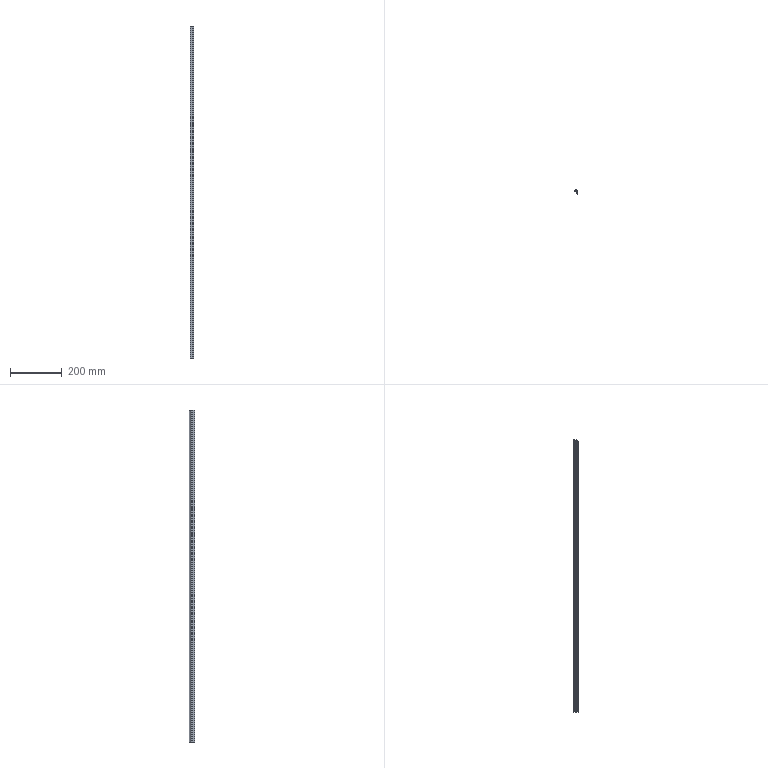Part | SolidWorks | features BaseBody 1, ICE 1, MoveFace 1 | 1 solid | 27 faces | box 14 x 20.3 x 1280 mm | volume 65172 mm3 | plane 20 | cylinder 7 | commonest cylinder face diameters 0.387 x2 0.8 x2 0.4 x1 20 x1 22 x1
STEP:
#1=CARTESIAN_POINT('',(-5.304,-0.625,200.));
#2=VERTEX_POINT('',#1);
#3=CARTESIAN_POINT('',(-5.449,-0.8125,200.));
#4=VERTEX_POINT('',#3);
#5=CARTESIAN_POINT('',(-5.255,-0.8125,200.));
#6=DIRECTION('',(0.,0.,1.));
#7=DIRECTION('',(-1.,0.,0.));
#8=AXIS2_PLACEMENT_3D('',#5,#6,#7);
#9=CIRCLE('',#8,0.1937);
#10=EDGE_CURVE('',#2,#4,#9,.T.);
#11=ORIENTED_EDGE('',*,*,#10,.T.);
#12=CARTESIAN_POINT('',(-5.449,-0.8125,-1080.));
#13=VERTEX_POINT('',#12);
#14=CARTESIAN_POINT('',(-5.449,-0.8125,230.));
#15=DIRECTION('',(0.,0.,-1.));
#16=VECTOR('',#15,1000.);
#17=LINE('',#14,#16);
#18=EDGE_CURVE('',#4,#13,#17,.T.);
#19=ORIENTED_EDGE('',*,*,#18,.T.);
#20=CARTESIAN_POINT('',(-5.304,-0.625,-1080.));
#21=VERTEX_POINT('',#20);
#22=CARTESIAN_POINT('',(-5.255,-0.8125,-1080.));
#23=DIRECTION('',(0.,0.,-1.));
#24=DIRECTION('',(1.,0.,0.));
#25=AXIS2_PLACEMENT_3D('',#22,#23,#24);
#26=CIRCLE('',#25,0.1937);
#27=EDGE_CURVE('',#13,#21,#26,.T.);
#28=ORIENTED_EDGE('',*,*,#27,.T.);
#29=CARTESIAN_POINT('',(-5.304,-0.625,230.));
#30=DIRECTION('',(0.,0.,-1.));
#31=VECTOR('',#30,1000.);
#32=LINE('',#29,#31);
#33=EDGE_CURVE('',#2,#21,#32,.T.);
#34=ORIENTED_EDGE('',*,*,#33,.F.);
#35=EDGE_LOOP('',(#11,#19,#28,#34));
#36=FACE_OUTER_BOUND('',#35,.T.);
#37=CARTESIAN_POINT('',(-5.255,-0.8125,230.));
#38=DIRECTION('',(0.,0.,-1.));
#39=DIRECTION('',(-1.,0.,0.));
#40=AXIS2_PLACEMENT_3D('',#37,#38,#39);
#41=CYLINDRICAL_SURFACE('',#40,0.1937);
#42=ADVANCED_FACE('',(#36),#41,.F.);
#43=CARTESIAN_POINT('',(5.,-1.,-1080.));
#44=VERTEX_POINT('',#43);
#45=CARTESIAN_POINT('',(5.,-14.3,-1080.));
#46=VERTEX_POINT('',#45);
#47=CARTESIAN_POINT('',(5.,29.623,-1080.));
#48=DIRECTION('',(0.,-1.,0.));
#49=VECTOR('',#48,1000.);
#50=LINE('',#47,#49);
#51=EDGE_CURVE('',#44,#46,#50,.T.);
#52=ORIENTED_EDGE('',*,*,#51,.F.);
#53=CARTESIAN_POINT('',(5.,-1.,200.));
#54=VERTEX_POINT('',#53);
#55=CARTESIAN_POINT('',(5.,-1.,230.));
#56=DIRECTION('',(0.,0.,-1.));
#57=VECTOR('',#56,1000.);
#58=LINE('',#55,#57);
#59=EDGE_CURVE('',#54,#44,#58,.T.);
#60=ORIENTED_EDGE('',*,*,#59,.F.);
#61=CARTESIAN_POINT('',(5.,-14.3,200.));
#62=VERTEX_POINT('',#61);
#63=CARTESIAN_POINT('',(5.,-14.3,200.));
#64=DIRECTION('',(0.,1.,0.));
#65=VECTOR('',#64,1000.);
#66=LINE('',#63,#65);
#67=EDGE_CURVE('',#62,#54,#66,.T.);
#68=ORIENTED_EDGE('',*,*,#67,.F.);
#69=CARTESIAN_POINT('',(5.,-14.3,230.));
#70=DIRECTION('',(0.,0.,1.));
#71=VECTOR('',#70,1000.);
#72=LINE('',#69,#71);
#73=EDGE_CURVE('',#46,#62,#72,.T.);
#74=ORIENTED_EDGE('',*,*,#73,.F.);
#75=EDGE_LOOP('',(#52,#60,#68,#74));
#76=FACE_OUTER_BOUND('',#75,.T.);
#77=CARTESIAN_POINT('',(5.,-14.3,230.));
#78=DIRECTION('',(-1.,0.,0.));
#79=DIRECTION('',(0.,0.,1.));
#80=AXIS2_PLACEMENT_3D('',#77,#78,#79);
#81=PLANE('',#80);
#82=ADVANCED_FACE('',(#76),#81,.F.);
#83=CARTESIAN_POINT('',(-9.,-2.,-1080.));
#84=VERTEX_POINT('',#83);
#85=CARTESIAN_POINT('',(-9.,-2.,200.));
#86=VERTEX_POINT('',#85);
#87=CARTESIAN_POINT('',(-9.,-2.,230.));
#88=DIRECTION('',(0.,0.,1.));
#89=VECTOR('',#88,1000.);
#90=LINE('',#87,#89);
#91=EDGE_CURVE('',#84,#86,#90,.T.);
#92=ORIENTED_EDGE('',*,*,#91,.F.);
#93=CARTESIAN_POINT('',(0.9,-2.,-1080.));
#94=VERTEX_POINT('',#93);
#95=CARTESIAN_POINT('',(5.,-2.,-1080.));
#96=DIRECTION('',(-1.,0.,0.));
#97=VECTOR('',#96,1000.);
#98=LINE('',#95,#97);
#99=EDGE_CURVE('',#94,#84,#98,.T.);
#100=ORIENTED_EDGE('',*,*,#99,.F.);
#101=CARTESIAN_POINT('',(0.9,-2.,200.));
#102=VERTEX_POINT('',#101);
#103=CARTESIAN_POINT('',(0.9,-2.,230.));
#104=DIRECTION('',(0.,0.,-1.));
#105=VECTOR('',#104,1000.);
#106=LINE('',#103,#105);
#107=EDGE_CURVE('',#102,#94,#106,.T.);
#108=ORIENTED_EDGE('',*,*,#107,.F.);
#109=CARTESIAN_POINT('',(5.,-2.,200.));
#110=DIRECTION('',(1.,0.,0.));
#111=VECTOR('',#110,1000.);
#112=LINE('',#109,#111);
#113=EDGE_CURVE('',#86,#102,#112,.T.);
#114=ORIENTED_EDGE('',*,*,#113,.F.);
#115=EDGE_LOOP('',(#92,#100,#108,#114));
#116=FACE_OUTER_BOUND('',#115,.T.);
#117=CARTESIAN_POINT('',(-9.,-2.,230.));
#118=DIRECTION('',(0.,1.,0.));
#119=DIRECTION('',(0.,0.,1.));
#120=AXIS2_PLACEMENT_3D('',#117,#118,#119);
#121=PLANE('',#120);
#122=ADVANCED_FACE('',(#116),#121,.F.);
#123=CARTESIAN_POINT('',(4.,-6.,200.));
#124=VERTEX_POINT('',#123);
#125=CARTESIAN_POINT('',(4.,-3.,200.));
#126=VERTEX_POINT('',#125);
#127=CARTESIAN_POINT('',(4.,29.623,200.));
#128=DIRECTION('',(0.,1.,0.));
#129=VECTOR('',#128,1000.);
#130=LINE('',#127,#129);
#131=EDGE_CURVE('',#124,#126,#130,.T.);
#132=ORIENTED_EDGE('',*,*,#131,.F.);
#133=CARTESIAN_POINT('',(1.,-6.,200.));
#134=VERTEX_POINT('',#133);
#135=CARTESIAN_POINT('',(5.,-6.,200.));
#136=DIRECTION('',(1.,0.,0.));
#137=VECTOR('',#136,1000.);
#138=LINE('',#135,#137);
#139=EDGE_CURVE('',#134,#124,#138,.T.);
#140=ORIENTED_EDGE('',*,*,#139,.F.);
#141=CARTESIAN_POINT('',(1.,-6.7,200.));
#142=VERTEX_POINT('',#141);
#143=CARTESIAN_POINT('',(1.,-6.,200.));
#144=DIRECTION('',(0.,-1.,0.));
#145=VECTOR('',#144,1000.);
#146=LINE('',#143,#145);
#147=EDGE_CURVE('',#134,#142,#146,.T.);
#148=ORIENTED_EDGE('',*,*,#147,.T.);
#149=CARTESIAN_POINT('',(-1.7,-6.7,200.));
#150=VERTEX_POINT('',#149);
#151=CARTESIAN_POINT('',(5.,-6.7,200.));
#152=DIRECTION('',(1.,0.,0.));
#153=VECTOR('',#152,1000.);
#154=LINE('',#151,#153);
#155=EDGE_CURVE('',#150,#142,#154,.T.);
#156=ORIENTED_EDGE('',*,*,#155,.F.);
#157=CARTESIAN_POINT('',(-1.7,-7.7,200.));
#158=VERTEX_POINT('',#157);
#159=CARTESIAN_POINT('',(-1.7,-6.7,200.));
#160=DIRECTION('',(0.,-1.,0.));
#161=VECTOR('',#160,1000.);
#162=LINE('',#159,#161);
#163=EDGE_CURVE('',#150,#158,#162,.T.);
#164=ORIENTED_EDGE('',*,*,#163,.T.);
#165=CARTESIAN_POINT('',(4.,-7.7,200.));
#166=VERTEX_POINT('',#165);
#167=CARTESIAN_POINT('',(5.,-7.7,200.));
#168=DIRECTION('',(-1.,0.,0.));
#169=VECTOR('',#168,1000.);
#170=LINE('',#167,#169);
#171=EDGE_CURVE('',#166,#158,#170,.T.);
#172=ORIENTED_EDGE('',*,*,#171,.F.);
#173=CARTESIAN_POINT('',(4.,-14.3,200.));
#174=VERTEX_POINT('',#173);
#175=CARTESIAN_POINT('',(4.,29.623,200.));
#176=DIRECTION('',(0.,1.,0.));
#177=VECTOR('',#176,1000.);
#178=LINE('',#175,#177);
#179=EDGE_CURVE('',#174,#166,#178,.T.);
#180=ORIENTED_EDGE('',*,*,#179,.F.);
#181=CARTESIAN_POINT('',(5.,-14.3,200.));
#182=DIRECTION('',(-1.,0.,0.));
#183=VECTOR('',#182,1000.);
#184=LINE('',#181,#183);
#185=EDGE_CURVE('',#62,#174,#184,.T.);
#186=ORIENTED_EDGE('',*,*,#185,.F.);
#187=ORIENTED_EDGE('',*,*,#67,.T.);
#188=CARTESIAN_POINT('',(-5.207,-1.,200.));
#189=VERTEX_POINT('',#188);
#190=CARTESIAN_POINT('',(5.,-1.,200.));
#191=DIRECTION('',(1.,0.,0.));
#192=VECTOR('',#191,1000.);
#193=LINE('',#190,#192);
#194=EDGE_CURVE('',#189,#54,#193,.T.);
#195=ORIENTED_EDGE('',*,*,#194,.F.);
#196=CARTESIAN_POINT('',(-5.255,-0.8125,200.));
#197=DIRECTION('',(0.,0.,1.));
#198=DIRECTION('',(-1.,0.,0.));
#199=AXIS2_PLACEMENT_3D('',#196,#197,#198);
#200=CIRCLE('',#199,0.1937);
#201=EDGE_CURVE('',#4,#189,#200,.T.);
#202=ORIENTED_EDGE('',*,*,#201,.F.);
#203=ORIENTED_EDGE('',*,*,#10,.F.);
#204=CARTESIAN_POINT('',(-1.368,3.063,200.));
#205=VERTEX_POINT('',#204);
#206=CARTESIAN_POINT('',(-10.628,9.,200.));
#207=DIRECTION('',(0.,0.,1.));
#208=DIRECTION('',(-1.,0.,0.));
#209=AXIS2_PLACEMENT_3D('',#206,#207,#208);
#210=CIRCLE('',#209,11.);
#211=EDGE_CURVE('',#2,#205,#210,.T.);
#212=ORIENTED_EDGE('',*,*,#211,.T.);
#213=CARTESIAN_POINT('',(-1.,2.955,200.));
#214=VERTEX_POINT('',#213);
#215=CARTESIAN_POINT('',(-1.2,2.955,200.));
#216=DIRECTION('',(0.,0.,1.));
#217=DIRECTION('',(-1.,0.,0.));
#218=AXIS2_PLACEMENT_3D('',#215,#216,#217);
#219=CIRCLE('',#218,0.2);
#220=EDGE_CURVE('',#214,#205,#219,.T.);
#221=ORIENTED_EDGE('',*,*,#220,.F.);
#222=CARTESIAN_POINT('',(-1.,1.5,200.));
#223=VERTEX_POINT('',#222);
#224=CARTESIAN_POINT('',(-1.,2.955,200.));
#225=DIRECTION('',(0.,1.,0.));
#226=VECTOR('',#225,1000.);
#227=LINE('',#224,#226);
#228=EDGE_CURVE('',#223,#214,#227,.T.);
#229=ORIENTED_EDGE('',*,*,#228,.F.);
#230=CARTESIAN_POINT('',(0.,1.5,200.));
#231=VERTEX_POINT('',#230);
#232=CARTESIAN_POINT('',(-1.,1.5,200.));
#233=DIRECTION('',(-1.,0.,0.));
#234=VECTOR('',#233,1000.);
#235=LINE('',#232,#234);
#236=EDGE_CURVE('',#231,#223,#235,.T.);
#237=ORIENTED_EDGE('',*,*,#236,.F.);
#238=CARTESIAN_POINT('',(0.,6.,200.));
#239=VERTEX_POINT('',#238);
#240=CARTESIAN_POINT('',(0.,1.5,200.));
#241=DIRECTION('',(0.,-1.,0.));
#242=VECTOR('',#241,1000.);
#243=LINE('',#240,#242);
#244=EDGE_CURVE('',#239,#231,#243,.T.);
#245=ORIENTED_EDGE('',*,*,#244,.F.);
#246=CARTESIAN_POINT('',(-0.8,6.,200.));
#247=VERTEX_POINT('',#246);
#248=CARTESIAN_POINT('',(0.,6.,200.));
#249=DIRECTION('',(1.,0.,0.));
#250=VECTOR('',#249,1000.);
#251=LINE('',#248,#250);
#252=EDGE_CURVE('',#247,#239,#251,.T.);
#253=ORIENTED_EDGE('',*,*,#252,.F.);
#254=CARTESIAN_POINT('',(-1.178,5.731,200.));
#255=VERTEX_POINT('',#254);
#256=CARTESIAN_POINT('',(-0.8,5.6,200.));
#257=DIRECTION('',(0.,0.,1.));
#258=DIRECTION('',(-1.,0.,0.));
#259=AXIS2_PLACEMENT_3D('',#256,#257,#258);
#260=CIRCLE('',#259,0.4);
#261=EDGE_CURVE('',#247,#255,#260,.T.);
#262=ORIENTED_EDGE('',*,*,#261,.T.);
#263=CARTESIAN_POINT('',(-8.678,-0.8077,200.));
#264=VERTEX_POINT('',#263);
#265=CARTESIAN_POINT('',(-10.628,9.,200.));
#266=DIRECTION('',(0.,0.,1.));
#267=DIRECTION('',(-1.,0.,0.));
#268=AXIS2_PLACEMENT_3D('',#265,#266,#267);
#269=CIRCLE('',#268,10.);
#270=EDGE_CURVE('',#264,#255,#269,.T.);
#271=ORIENTED_EDGE('',*,*,#270,.F.);
#272=CARTESIAN_POINT('',(-9.,-1.2,200.));
#273=VERTEX_POINT('',#272);
#274=CARTESIAN_POINT('',(-8.6,-1.2,200.));
#275=DIRECTION('',(0.,0.,1.));
#276=DIRECTION('',(-1.,0.,0.));
#277=AXIS2_PLACEMENT_3D('',#274,#275,#276);
#278=CIRCLE('',#277,0.4);
#279=EDGE_CURVE('',#264,#273,#278,.T.);
#280=ORIENTED_EDGE('',*,*,#279,.T.);
#281=CARTESIAN_POINT('',(-9.,8.,200.));
#282=DIRECTION('',(0.,-1.,0.));
#283=VECTOR('',#282,1000.);
#284=LINE('',#281,#283);
#285=EDGE_CURVE('',#273,#86,#284,.T.);
#286=ORIENTED_EDGE('',*,*,#285,.T.);
#287=ORIENTED_EDGE('',*,*,#113,.T.);
#288=CARTESIAN_POINT('',(0.9,-3.,200.));
#289=VERTEX_POINT('',#288);
#290=CARTESIAN_POINT('',(0.9,29.623,200.));
#291=DIRECTION('',(0.,1.,0.));
#292=VECTOR('',#291,1000.);
#293=LINE('',#290,#292);
#294=EDGE_CURVE('',#289,#102,#293,.T.);
#295=ORIENTED_EDGE('',*,*,#294,.F.);
#296=CARTESIAN_POINT('',(5.,-3.,200.));
#297=DIRECTION('',(-1.,0.,0.));
#298=VECTOR('',#297,1000.);
#299=LINE('',#296,#298);
#300=EDGE_CURVE('',#126,#289,#299,.T.);
#301=ORIENTED_EDGE('',*,*,#300,.F.);
#302=EDGE_LOOP('',(#132,#140,#148,#156,#164,#172,#180,#186,#187,#195,#202,#203,#212,#221,#229,#237,#245,#253,#262,#271,#280,#286,#287,#295,#301));
#303=FACE_OUTER_BOUND('',#302,.T.);
#304=CARTESIAN_POINT('',(5.,29.623,200.));
#305=DIRECTION('',(0.,0.,-1.));
#306=DIRECTION('',(-1.,0.,0.));
#307=AXIS2_PLACEMENT_3D('',#304,#305,#306);
#308=PLANE('',#307);
#309=ADVANCED_FACE('',(#303),#308,.F.);
#310=ORIENTED_EDGE('',*,*,#185,.T.);
#311=CARTESIAN_POINT('',(4.,-14.3,-1080.));
#312=VERTEX_POINT('',#311);
#313=CARTESIAN_POINT('',(4.,-14.3,230.));
#314=DIRECTION('',(0.,0.,1.));
#315=VECTOR('',#314,1000.);
#316=LINE('',#313,#315);
#317=EDGE_CURVE('',#312,#174,#316,.T.);
#318=ORIENTED_EDGE('',*,*,#317,.F.);
#319=CARTESIAN_POINT('',(5.,-14.3,-1080.));
#320=DIRECTION('',(-1.,0.,0.));
#321=VECTOR('',#320,1000.);
#322=LINE('',#319,#321);
#323=EDGE_CURVE('',#46,#312,#322,.T.);
#324=ORIENTED_EDGE('',*,*,#323,.F.);
#325=ORIENTED_EDGE('',*,*,#73,.T.);
#326=EDGE_LOOP('',(#310,#318,#324,#325));
#327=FACE_OUTER_BOUND('',#326,.T.);
#328=CARTESIAN_POINT('',(4.,-14.3,230.));
#329=DIRECTION('',(0.,1.,0.));
#330=DIRECTION('',(0.,0.,1.));
#331=AXIS2_PLACEMENT_3D('',#328,#329,#330);
#332=PLANE('',#331);
#333=ADVANCED_FACE('',(#327),#332,.F.);
#334=ORIENTED_EDGE('',*,*,#51,.T.);
#335=ORIENTED_EDGE('',*,*,#323,.T.);
#336=CARTESIAN_POINT('',(4.,-7.7,-1080.));
#337=VERTEX_POINT('',#336);
#338=CARTESIAN_POINT('',(4.,-7.7,-1080.));
#339=DIRECTION('',(0.,-1.,0.));
#340=VECTOR('',#339,1000.);
#341=LINE('',#338,#340);
#342=EDGE_CURVE('',#337,#312,#341,.T.);
#343=ORIENTED_EDGE('',*,*,#342,.F.);
#344=CARTESIAN_POINT('',(-1.7,-7.7,-1080.));
#345=VERTEX_POINT('',#344);
#346=CARTESIAN_POINT('',(-1.7,-7.7,-1080.));
#347=DIRECTION('',(1.,0.,0.));
#348=VECTOR('',#347,1000.);
#349=LINE('',#346,#348);
#350=EDGE_CURVE('',#345,#337,#349,.T.);
#351=ORIENTED_EDGE('',*,*,#350,.F.);
#352=CARTESIAN_POINT('',(-1.7,-6.7,-1080.));
#353=VERTEX_POINT('',#352);
#354=CARTESIAN_POINT('',(-1.7,29.623,-1080.));
#355=DIRECTION('',(0.,1.,0.));
#356=VECTOR('',#355,1000.);
#357=LINE('',#354,#356);
#358=EDGE_CURVE('',#345,#353,#357,.T.);
#359=ORIENTED_EDGE('',*,*,#358,.T.);
#360=CARTESIAN_POINT('',(1.,-6.7,-1080.));
#361=VERTEX_POINT('',#360);
#362=CARTESIAN_POINT('',(1.,-6.7,-1080.));
#363=DIRECTION('',(-1.,0.,0.));
#364=VECTOR('',#363,1000.);
#365=LINE('',#362,#364);
#366=EDGE_CURVE('',#361,#353,#365,.T.);
#367=ORIENTED_EDGE('',*,*,#366,.F.);
#368=CARTESIAN_POINT('',(1.,-6.,-1080.));
#369=VERTEX_POINT('',#368);
#370=CARTESIAN_POINT('',(1.,29.623,-1080.));
#371=DIRECTION('',(0.,1.,0.));
#372=VECTOR('',#371,1000.);
#373=LINE('',#370,#372);
#374=EDGE_CURVE('',#361,#369,#373,.T.);
#375=ORIENTED_EDGE('',*,*,#374,.T.);
#376=CARTESIAN_POINT('',(4.,-6.,-1080.));
#377=VERTEX_POINT('',#376);
#378=CARTESIAN_POINT('',(4.,-6.,-1080.));
#379=DIRECTION('',(-1.,0.,0.));
#380=VECTOR('',#379,1000.);
#381=LINE('',#378,#380);
#382=EDGE_CURVE('',#377,#369,#381,.T.);
#383=ORIENTED_EDGE('',*,*,#382,.F.);
#384=CARTESIAN_POINT('',(4.,-3.,-1080.));
#385=VERTEX_POINT('',#384);
#386=CARTESIAN_POINT('',(4.,-3.,-1080.));
#387=DIRECTION('',(0.,-1.,0.));
#388=VECTOR('',#387,1000.);
#389=LINE('',#386,#388);
#390=EDGE_CURVE('',#385,#377,#389,.T.);
#391=ORIENTED_EDGE('',*,*,#390,.F.);
#392=CARTESIAN_POINT('',(0.9,-3.,-1080.));
#393=VERTEX_POINT('',#392);
#394=CARTESIAN_POINT('',(0.9,-3.,-1080.));
#395=DIRECTION('',(1.,0.,0.));
#396=VECTOR('',#395,1000.);
#397=LINE('',#394,#396);
#398=EDGE_CURVE('',#393,#385,#397,.T.);
#399=ORIENTED_EDGE('',*,*,#398,.F.);
#400=CARTESIAN_POINT('',(0.9,-2.,-1080.));
#401=DIRECTION('',(0.,-1.,0.));
#402=VECTOR('',#401,1000.);
#403=LINE('',#400,#402);
#404=EDGE_CURVE('',#94,#393,#403,.T.);
#405=ORIENTED_EDGE('',*,*,#404,.F.);
#406=ORIENTED_EDGE('',*,*,#99,.T.);
#407=CARTESIAN_POINT('',(-9.,-1.2,-1080.));
#408=VERTEX_POINT('',#407);
#409=CARTESIAN_POINT('',(-9.,-1.2,-1080.));
#410=DIRECTION('',(0.,-1.,0.));
#411=VECTOR('',#410,1000.);
#412=LINE('',#409,#411);
#413=EDGE_CURVE('',#408,#84,#412,.T.);
#414=ORIENTED_EDGE('',*,*,#413,.F.);
#415=CARTESIAN_POINT('',(-8.678,-0.8077,-1080.));
#416=VERTEX_POINT('',#415);
#417=CARTESIAN_POINT('',(-8.6,-1.2,-1080.));
#418=DIRECTION('',(0.,0.,-1.));
#419=DIRECTION('',(1.,0.,0.));
#420=AXIS2_PLACEMENT_3D('',#417,#418,#419);
#421=CIRCLE('',#420,0.4);
#422=EDGE_CURVE('',#408,#416,#421,.T.);
#423=ORIENTED_EDGE('',*,*,#422,.T.);
#424=CARTESIAN_POINT('',(-1.178,5.731,-1080.));
#425=VERTEX_POINT('',#424);
#426=CARTESIAN_POINT('',(-10.628,9.,-1080.));
#427=DIRECTION('',(0.,0.,-1.));
#428=DIRECTION('',(1.,0.,0.));
#429=AXIS2_PLACEMENT_3D('',#426,#427,#428);
#430=CIRCLE('',#429,10.);
#431=EDGE_CURVE('',#425,#416,#430,.T.);
#432=ORIENTED_EDGE('',*,*,#431,.F.);
#433=CARTESIAN_POINT('',(-0.8,6.,-1080.));
#434=VERTEX_POINT('',#433);
#435=CARTESIAN_POINT('',(-0.8,5.6,-1080.));
#436=DIRECTION('',(0.,0.,-1.));
#437=DIRECTION('',(1.,0.,0.));
#438=AXIS2_PLACEMENT_3D('',#435,#436,#437);
#439=CIRCLE('',#438,0.4);
#440=EDGE_CURVE('',#425,#434,#439,.T.);
#441=ORIENTED_EDGE('',*,*,#440,.T.);
#442=CARTESIAN_POINT('',(0.,6.,-1080.));
#443=VERTEX_POINT('',#442);
#444=CARTESIAN_POINT('',(0.,6.,-1080.));
#445=DIRECTION('',(-1.,0.,0.));
#446=VECTOR('',#445,1000.);
#447=LINE('',#444,#446);
#448=EDGE_CURVE('',#443,#434,#447,.T.);
#449=ORIENTED_EDGE('',*,*,#448,.F.);
#450=CARTESIAN_POINT('',(0.,1.5,-1080.));
#451=VERTEX_POINT('',#450);
#452=CARTESIAN_POINT('',(0.,1.5,-1080.));
#453=DIRECTION('',(0.,1.,0.));
#454=VECTOR('',#453,1000.);
#455=LINE('',#452,#454);
#456=EDGE_CURVE('',#451,#443,#455,.T.);
#457=ORIENTED_EDGE('',*,*,#456,.F.);
#458=CARTESIAN_POINT('',(-1.,1.5,-1080.));
#459=VERTEX_POINT('',#458);
#460=CARTESIAN_POINT('',(-1.,1.5,-1080.));
#461=DIRECTION('',(1.,0.,0.));
#462=VECTOR('',#461,1000.);
#463=LINE('',#460,#462);
#464=EDGE_CURVE('',#459,#451,#463,.T.);
#465=ORIENTED_EDGE('',*,*,#464,.F.);
#466=CARTESIAN_POINT('',(-1.,2.955,-1080.));
#467=VERTEX_POINT('',#466);
#468=CARTESIAN_POINT('',(-1.,2.955,-1080.));
#469=DIRECTION('',(0.,-1.,0.));
#470=VECTOR('',#469,1000.);
#471=LINE('',#468,#470);
#472=EDGE_CURVE('',#467,#459,#471,.T.);
#473=ORIENTED_EDGE('',*,*,#472,.F.);
#474=CARTESIAN_POINT('',(-1.368,3.063,-1080.));
#475=VERTEX_POINT('',#474);
#476=CARTESIAN_POINT('',(-1.2,2.955,-1080.));
#477=DIRECTION('',(0.,0.,-1.));
#478=DIRECTION('',(1.,0.,0.));
#479=AXIS2_PLACEMENT_3D('',#476,#477,#478);
#480=CIRCLE('',#479,0.2);
#481=EDGE_CURVE('',#475,#467,#480,.T.);
#482=ORIENTED_EDGE('',*,*,#481,.F.);
#483=CARTESIAN_POINT('',(-10.628,9.,-1080.));
#484=DIRECTION('',(0.,0.,-1.));
#485=DIRECTION('',(1.,0.,0.));
#486=AXIS2_PLACEMENT_3D('',#483,#484,#485);
#487=CIRCLE('',#486,11.);
#488=EDGE_CURVE('',#475,#21,#487,.T.);
#489=ORIENTED_EDGE('',*,*,#488,.T.);
#490=ORIENTED_EDGE('',*,*,#27,.F.);
#491=CARTESIAN_POINT('',(-5.207,-1.,-1080.));
#492=VERTEX_POINT('',#491);
#493=CARTESIAN_POINT('',(-5.255,-0.8125,-1080.));
#494=DIRECTION('',(0.,0.,-1.));
#495=DIRECTION('',(1.,0.,0.));
#496=AXIS2_PLACEMENT_3D('',#493,#494,#495);
#497=CIRCLE('',#496,0.1937);
#498=EDGE_CURVE('',#492,#13,#497,.T.);
#499=ORIENTED_EDGE('',*,*,#498,.F.);
#500=CARTESIAN_POINT('',(5.,-1.,-1080.));
#501=DIRECTION('',(-1.,0.,0.));
#502=VECTOR('',#501,1000.);
#503=LINE('',#500,#502);
#504=EDGE_CURVE('',#44,#492,#503,.T.);
#505=ORIENTED_EDGE('',*,*,#504,.F.);
#506=EDGE_LOOP('',(#334,#335,#343,#351,#359,#367,#375,#383,#391,#399,#405,#406,#414,#423,#432,#441,#449,#457,#465,#473,#482,#489,#490,#499,#505));
#507=FACE_OUTER_BOUND('',#506,.T.);
#508=CARTESIAN_POINT('',(5.,29.623,-1080.));
#509=DIRECTION('',(0.,0.,1.));
#510=DIRECTION('',(1.,0.,0.));
#511=AXIS2_PLACEMENT_3D('',#508,#509,#510);
#512=PLANE('',#511);
#513=ADVANCED_FACE('',(#507),#512,.F.);
#514=ORIENTED_EDGE('',*,*,#59,.T.);
#515=ORIENTED_EDGE('',*,*,#504,.T.);
#516=CARTESIAN_POINT('',(-5.207,-1.,230.));
#517=DIRECTION('',(0.,0.,-1.));
#518=VECTOR('',#517,1000.);
#519=LINE('',#516,#518);
#520=EDGE_CURVE('',#189,#492,#519,.T.);
#521=ORIENTED_EDGE('',*,*,#520,.F.);
#522=ORIENTED_EDGE('',*,*,#194,.T.);
#523=EDGE_LOOP('',(#514,#515,#521,#522));
#524=FACE_OUTER_BOUND('',#523,.T.);
#525=CARTESIAN_POINT('',(5.,-1.,230.));
#526=DIRECTION('',(0.,-1.,0.));
#527=DIRECTION('',(0.,0.,-1.));
#528=AXIS2_PLACEMENT_3D('',#525,#526,#527);
#529=PLANE('',#528);
#530=ADVANCED_FACE('',(#524),#529,.F.);
#531=CARTESIAN_POINT('',(-9.,-1.2,230.));
#532=DIRECTION('',(0.,0.,1.));
#533=VECTOR('',#532,1000.);
#534=LINE('',#531,#533);
#535=EDGE_CURVE('',#408,#273,#534,.T.);
#536=ORIENTED_EDGE('',*,*,#535,.F.);
#537=ORIENTED_EDGE('',*,*,#413,.T.);
#538=ORIENTED_EDGE('',*,*,#91,.T.);
#539=ORIENTED_EDGE('',*,*,#285,.F.);
#540=EDGE_LOOP('',(#536,#537,#538,#539));
#541=FACE_OUTER_BOUND('',#540,.T.);
#542=CARTESIAN_POINT('',(-9.,-1.2,230.));
#543=DIRECTION('',(1.,0.,0.));
#544=DIRECTION('',(0.,0.,-1.));
#545=AXIS2_PLACEMENT_3D('',#542,#543,#544);
#546=PLANE('',#545);
#547=ADVANCED_FACE('',(#541),#546,.F.);
#548=ORIENTED_EDGE('',*,*,#294,.T.);
#549=ORIENTED_EDGE('',*,*,#107,.T.);
#550=ORIENTED_EDGE('',*,*,#404,.T.);
#551=CARTESIAN_POINT('',(0.9,-3.,230.));
#552=DIRECTION('',(0.,0.,-1.));
#553=VECTOR('',#552,1000.);
#554=LINE('',#551,#553);
#555=EDGE_CURVE('',#289,#393,#554,.T.);
#556=ORIENTED_EDGE('',*,*,#555,.F.);
#557=EDGE_LOOP('',(#548,#549,#550,#556));
#558=FACE_OUTER_BOUND('',#557,.T.);
#559=CARTESIAN_POINT('',(0.9,-2.,230.));
#560=DIRECTION('',(1.,0.,0.));
#561=DIRECTION('',(0.,0.,-1.));
#562=AXIS2_PLACEMENT_3D('',#559,#560,#561);
#563=PLANE('',#562);
#564=ADVANCED_FACE('',(#558),#563,.F.);
#565=ORIENTED_EDGE('',*,*,#300,.T.);
#566=ORIENTED_EDGE('',*,*,#555,.T.);
#567=ORIENTED_EDGE('',*,*,#398,.T.);
#568=CARTESIAN_POINT('',(4.,-3.,230.));
#569=DIRECTION('',(0.,0.,-1.));
#570=VECTOR('',#569,1000.);
#571=LINE('',#568,#570);
#572=EDGE_CURVE('',#126,#385,#571,.T.);
#573=ORIENTED_EDGE('',*,*,#572,.F.);
#574=EDGE_LOOP('',(#565,#566,#567,#573));
#575=FACE_OUTER_BOUND('',#574,.T.);
#576=CARTESIAN_POINT('',(0.9,-3.,230.));
#577=DIRECTION('',(0.,1.,0.));
#578=DIRECTION('',(0.,0.,1.));
#579=AXIS2_PLACEMENT_3D('',#576,#577,#578);
#580=PLANE('',#579);
#581=ADVANCED_FACE('',(#575),#580,.F.);
#582=ORIENTED_EDGE('',*,*,#131,.T.);
#583=ORIENTED_EDGE('',*,*,#572,.T.);
#584=ORIENTED_EDGE('',*,*,#390,.T.);
#585=CARTESIAN_POINT('',(4.,-6.,230.));
#586=DIRECTION('',(0.,0.,-1.));
#587=VECTOR('',#586,1000.);
#588=LINE('',#585,#587);
#589=EDGE_CURVE('',#124,#377,#588,.T.);
#590=ORIENTED_EDGE('',*,*,#589,.F.);
#591=EDGE_LOOP('',(#582,#583,#584,#590));
#592=FACE_OUTER_BOUND('',#591,.T.);
#593=CARTESIAN_POINT('',(4.,-3.,230.));
#594=DIRECTION('',(1.,0.,0.));
#595=DIRECTION('',(0.,0.,-1.));
#596=AXIS2_PLACEMENT_3D('',#593,#594,#595);
#597=PLANE('',#596);
#598=ADVANCED_FACE('',(#592),#597,.F.);
#599=ORIENTED_EDGE('',*,*,#139,.T.);
#600=ORIENTED_EDGE('',*,*,#589,.T.);
#601=ORIENTED_EDGE('',*,*,#382,.T.);
#602=CARTESIAN_POINT('',(1.,-6.,230.));
#603=DIRECTION('',(0.,0.,-1.));
#604=VECTOR('',#603,1000.);
#605=LINE('',#602,#604);
#606=EDGE_CURVE('',#134,#369,#605,.T.);
#607=ORIENTED_EDGE('',*,*,#606,.F.);
#608=EDGE_LOOP('',(#599,#600,#601,#607));
#609=FACE_OUTER_BOUND('',#608,.T.);
#610=CARTESIAN_POINT('',(4.,-6.,230.));
#611=DIRECTION('',(0.,-1.,0.));
#612=DIRECTION('',(0.,0.,-1.));
#613=AXIS2_PLACEMENT_3D('',#610,#611,#612);
#614=PLANE('',#613);
#615=ADVANCED_FACE('',(#609),#614,.F.);
#616=ORIENTED_EDGE('',*,*,#155,.T.);
#617=CARTESIAN_POINT('',(1.,-6.7,230.));
#618=DIRECTION('',(0.,0.,1.));
#619=VECTOR('',#618,1000.);
#620=LINE('',#617,#619);
#621=EDGE_CURVE('',#361,#142,#620,.T.);
#622=ORIENTED_EDGE('',*,*,#621,.F.);
#623=ORIENTED_EDGE('',*,*,#366,.T.);
#624=CARTESIAN_POINT('',(-1.7,-6.7,230.));
#625=DIRECTION('',(0.,0.,-1.));
#626=VECTOR('',#625,1000.);
#627=LINE('',#624,#626);
#628=EDGE_CURVE('',#150,#353,#627,.T.);
#629=ORIENTED_EDGE('',*,*,#628,.F.);
#630=EDGE_LOOP('',(#616,#622,#623,#629));
#631=FACE_OUTER_BOUND('',#630,.T.);
#632=CARTESIAN_POINT('',(1.,-6.7,230.));
#633=DIRECTION('',(0.,-1.,0.));
#634=DIRECTION('',(0.,0.,-1.));
#635=AXIS2_PLACEMENT_3D('',#632,#633,#634);
#636=PLANE('',#635);
#637=ADVANCED_FACE('',(#631),#636,.F.);
#638=ORIENTED_EDGE('',*,*,#171,.T.);
#639=CARTESIAN_POINT('',(-1.7,-7.7,230.));
#640=DIRECTION('',(0.,0.,1.));
#641=VECTOR('',#640,1000.);
#642=LINE('',#639,#641);
#643=EDGE_CURVE('',#345,#158,#642,.T.);
#644=ORIENTED_EDGE('',*,*,#643,.F.);
#645=ORIENTED_EDGE('',*,*,#350,.T.);
#646=CARTESIAN_POINT('',(4.,-7.7,230.));
#647=DIRECTION('',(0.,0.,-1.));
#648=VECTOR('',#647,1000.);
#649=LINE('',#646,#648);
#650=EDGE_CURVE('',#166,#337,#649,.T.);
#651=ORIENTED_EDGE('',*,*,#650,.F.);
#652=EDGE_LOOP('',(#638,#644,#645,#651));
#653=FACE_OUTER_BOUND('',#652,.T.);
#654=CARTESIAN_POINT('',(-1.7,-7.7,230.));
#655=DIRECTION('',(0.,1.,0.));
#656=DIRECTION('',(0.,0.,1.));
#657=AXIS2_PLACEMENT_3D('',#654,#655,#656);
#658=PLANE('',#657);
#659=ADVANCED_FACE('',(#653),#658,.F.);
#660=ORIENTED_EDGE('',*,*,#179,.T.);
#661=ORIENTED_EDGE('',*,*,#650,.T.);
#662=ORIENTED_EDGE('',*,*,#342,.T.);
#663=ORIENTED_EDGE('',*,*,#317,.T.);
#664=EDGE_LOOP('',(#660,#661,#662,#663));
#665=FACE_OUTER_BOUND('',#664,.T.);
#666=CARTESIAN_POINT('',(4.,-7.7,230.));
#667=DIRECTION('',(1.,0.,0.));
#668=DIRECTION('',(0.,0.,-1.));
#669=AXIS2_PLACEMENT_3D('',#666,#667,#668);
#670=PLANE('',#669);
#671=ADVANCED_FACE('',(#665),#670,.F.);
#672=ORIENTED_EDGE('',*,*,#18,.F.);
#673=ORIENTED_EDGE('',*,*,#201,.T.);
#674=ORIENTED_EDGE('',*,*,#520,.T.);
#675=ORIENTED_EDGE('',*,*,#498,.T.);
#676=EDGE_LOOP('',(#672,#673,#674,#675));
#677=FACE_OUTER_BOUND('',#676,.T.);
#678=CARTESIAN_POINT('',(-5.255,-0.8125,230.));
#679=DIRECTION('',(0.,0.,-1.));
#680=DIRECTION('',(-1.,0.,0.));
#681=AXIS2_PLACEMENT_3D('',#678,#679,#680);
#682=CYLINDRICAL_SURFACE('',#681,0.1937);
#683=ADVANCED_FACE('',(#677),#682,.F.);
#684=CARTESIAN_POINT('',(-1.,2.955,230.));
#685=DIRECTION('',(0.,0.,1.));
#686=VECTOR('',#685,1000.);
#687=LINE('',#684,#686);
#688=EDGE_CURVE('',#467,#214,#687,.T.);
#689=ORIENTED_EDGE('',*,*,#688,.F.);
#690=ORIENTED_EDGE('',*,*,#472,.T.);
#691=CARTESIAN_POINT('',(-1.,1.5,230.));
#692=DIRECTION('',(0.,0.,-1.));
#693=VECTOR('',#692,1000.);
#694=LINE('',#691,#693);
#695=EDGE_CURVE('',#223,#459,#694,.T.);
#696=ORIENTED_EDGE('',*,*,#695,.F.);
#697=ORIENTED_EDGE('',*,*,#228,.T.);
#698=EDGE_LOOP('',(#689,#690,#696,#697));
#699=FACE_OUTER_BOUND('',#698,.T.);
#700=CARTESIAN_POINT('',(-1.,2.955,230.));
#701=DIRECTION('',(1.,0.,0.));
#702=DIRECTION('',(0.,0.,-1.));
#703=AXIS2_PLACEMENT_3D('',#700,#701,#702);
#704=PLANE('',#703);
#705=ADVANCED_FACE('',(#699),#704,.F.);
#706=ORIENTED_EDGE('',*,*,#488,.F.);
#707=CARTESIAN_POINT('',(-1.368,3.063,230.));
#708=DIRECTION('',(0.,0.,1.));
#709=VECTOR('',#708,1000.);
#710=LINE('',#707,#709);
#711=EDGE_CURVE('',#475,#205,#710,.T.);
#712=ORIENTED_EDGE('',*,*,#711,.T.);
#713=ORIENTED_EDGE('',*,*,#211,.F.);
#714=ORIENTED_EDGE('',*,*,#33,.T.);
#715=EDGE_LOOP('',(#706,#712,#713,#714));
#716=FACE_OUTER_BOUND('',#715,.T.);
#717=CARTESIAN_POINT('',(-10.628,9.,230.));
#718=DIRECTION('',(0.,0.,-1.));
#719=DIRECTION('',(-1.,0.,0.));
#720=AXIS2_PLACEMENT_3D('',#717,#718,#719);
#721=CYLINDRICAL_SURFACE('',#720,11.);
#722=ADVANCED_FACE('',(#716),#721,.T.);
#723=CARTESIAN_POINT('',(-1.178,5.731,230.));
#724=DIRECTION('',(0.,0.,1.));
#725=VECTOR('',#724,1000.);
#726=LINE('',#723,#725);
#727=EDGE_CURVE('',#425,#255,#726,.T.);
#728=ORIENTED_EDGE('',*,*,#727,.F.);
#729=ORIENTED_EDGE('',*,*,#431,.T.);
#730=CARTESIAN_POINT('',(-8.678,-0.8077,230.));
#731=DIRECTION('',(0.,0.,-1.));
#732=VECTOR('',#731,1000.);
#733=LINE('',#730,#732);
#734=EDGE_CURVE('',#264,#416,#733,.T.);
#735=ORIENTED_EDGE('',*,*,#734,.F.);
#736=ORIENTED_EDGE('',*,*,#270,.T.);
#737=EDGE_LOOP('',(#728,#729,#735,#736));
#738=FACE_OUTER_BOUND('',#737,.T.);
#739=CARTESIAN_POINT('',(-10.628,9.,230.));
#740=DIRECTION('',(0.,0.,-1.));
#741=DIRECTION('',(-1.,0.,0.));
#742=AXIS2_PLACEMENT_3D('',#739,#740,#741);
#743=CYLINDRICAL_SURFACE('',#742,10.);
#744=ADVANCED_FACE('',(#738),#743,.F.);
#745=CARTESIAN_POINT('',(0.,1.5,230.));
#746=DIRECTION('',(0.,0.,1.));
#747=VECTOR('',#746,1000.);
#748=LINE('',#745,#747);
#749=EDGE_CURVE('',#451,#231,#748,.T.);
#750=ORIENTED_EDGE('',*,*,#749,.F.);
#751=ORIENTED_EDGE('',*,*,#456,.T.);
#752=CARTESIAN_POINT('',(0.,6.,230.));
#753=DIRECTION('',(0.,0.,-1.));
#754=VECTOR('',#753,1000.);
#755=LINE('',#752,#754);
#756=EDGE_CURVE('',#239,#443,#755,.T.);
#757=ORIENTED_EDGE('',*,*,#756,.F.);
#758=ORIENTED_EDGE('',*,*,#244,.T.);
#759=EDGE_LOOP('',(#750,#751,#757,#758));
#760=FACE_OUTER_BOUND('',#759,.T.);
#761=CARTESIAN_POINT('',(0.,1.5,230.));
#762=DIRECTION('',(-1.,0.,0.));
#763=DIRECTION('',(0.,0.,1.));
#764=AXIS2_PLACEMENT_3D('',#761,#762,#763);
#765=PLANE('',#764);
#766=ADVANCED_FACE('',(#760),#765,.F.);
#767=ORIENTED_EDGE('',*,*,#422,.F.);
#768=ORIENTED_EDGE('',*,*,#535,.T.);
#769=ORIENTED_EDGE('',*,*,#279,.F.);
#770=ORIENTED_EDGE('',*,*,#734,.T.);
#771=EDGE_LOOP('',(#767,#768,#769,#770));
#772=FACE_OUTER_BOUND('',#771,.T.);
#773=CARTESIAN_POINT('',(-8.6,-1.2,230.));
#774=DIRECTION('',(0.,0.,-1.));
#775=DIRECTION('',(-1.,0.,0.));
#776=AXIS2_PLACEMENT_3D('',#773,#774,#775);
#777=CYLINDRICAL_SURFACE('',#776,0.4);
#778=ADVANCED_FACE('',(#772),#777,.T.);
#779=ORIENTED_EDGE('',*,*,#147,.F.);
#780=ORIENTED_EDGE('',*,*,#606,.T.);
#781=ORIENTED_EDGE('',*,*,#374,.F.);
#782=ORIENTED_EDGE('',*,*,#621,.T.);
#783=EDGE_LOOP('',(#779,#780,#781,#782));
#784=FACE_OUTER_BOUND('',#783,.T.);
#785=CARTESIAN_POINT('',(1.,-6.,230.));
#786=DIRECTION('',(1.,0.,0.));
#787=DIRECTION('',(0.,0.,-1.));
#788=AXIS2_PLACEMENT_3D('',#785,#786,#787);
#789=PLANE('',#788);
#790=ADVANCED_FACE('',(#784),#789,.F.);
#791=ORIENTED_EDGE('',*,*,#163,.F.);
#792=ORIENTED_EDGE('',*,*,#628,.T.);
#793=ORIENTED_EDGE('',*,*,#358,.F.);
#794=ORIENTED_EDGE('',*,*,#643,.T.);
#795=EDGE_LOOP('',(#791,#792,#793,#794));
#796=FACE_OUTER_BOUND('',#795,.T.);
#797=CARTESIAN_POINT('',(-1.7,-6.7,230.));
#798=DIRECTION('',(1.,0.,0.));
#799=DIRECTION('',(0.,0.,-1.));
#800=AXIS2_PLACEMENT_3D('',#797,#798,#799);
#801=PLANE('',#800);
#802=ADVANCED_FACE('',(#796),#801,.F.);
#803=ORIENTED_EDGE('',*,*,#711,.F.);
#804=ORIENTED_EDGE('',*,*,#481,.T.);
#805=ORIENTED_EDGE('',*,*,#688,.T.);
#806=ORIENTED_EDGE('',*,*,#220,.T.);
#807=EDGE_LOOP('',(#803,#804,#805,#806));
#808=FACE_OUTER_BOUND('',#807,.T.);
#809=CARTESIAN_POINT('',(-1.2,2.955,230.));
#810=DIRECTION('',(0.,0.,-1.));
#811=DIRECTION('',(-1.,0.,0.));
#812=AXIS2_PLACEMENT_3D('',#809,#810,#811);
#813=CYLINDRICAL_SURFACE('',#812,0.2);
#814=ADVANCED_FACE('',(#808),#813,.F.);
#815=ORIENTED_EDGE('',*,*,#695,.T.);
#816=ORIENTED_EDGE('',*,*,#464,.T.);
#817=ORIENTED_EDGE('',*,*,#749,.T.);
#818=ORIENTED_EDGE('',*,*,#236,.T.);
#819=EDGE_LOOP('',(#815,#816,#817,#818));
#820=FACE_OUTER_BOUND('',#819,.T.);
#821=CARTESIAN_POINT('',(-1.,1.5,230.));
#822=DIRECTION('',(0.,1.,0.));
#823=DIRECTION('',(0.,0.,1.));
#824=AXIS2_PLACEMENT_3D('',#821,#822,#823);
#825=PLANE('',#824);
#826=ADVANCED_FACE('',(#820),#825,.F.);
#827=ORIENTED_EDGE('',*,*,#440,.F.);
#828=ORIENTED_EDGE('',*,*,#727,.T.);
#829=ORIENTED_EDGE('',*,*,#261,.F.);
#830=CARTESIAN_POINT('',(-0.8,6.,230.));
#831=DIRECTION('',(0.,0.,-1.));
#832=VECTOR('',#831,1000.);
#833=LINE('',#830,#832);
#834=EDGE_CURVE('',#247,#434,#833,.T.);
#835=ORIENTED_EDGE('',*,*,#834,.T.);
#836=EDGE_LOOP('',(#827,#828,#829,#835));
#837=FACE_OUTER_BOUND('',#836,.T.);
#838=CARTESIAN_POINT('',(-0.8,5.6,230.));
#839=DIRECTION('',(0.,0.,-1.));
#840=DIRECTION('',(-1.,0.,0.));
#841=AXIS2_PLACEMENT_3D('',#838,#839,#840);
#842=CYLINDRICAL_SURFACE('',#841,0.4);
#843=ADVANCED_FACE('',(#837),#842,.T.);
#844=ORIENTED_EDGE('',*,*,#756,.T.);
#845=ORIENTED_EDGE('',*,*,#448,.T.);
#846=ORIENTED_EDGE('',*,*,#834,.F.);
#847=ORIENTED_EDGE('',*,*,#252,.T.);
#848=EDGE_LOOP('',(#844,#845,#846,#847));
#849=FACE_OUTER_BOUND('',#848,.T.);
#850=CARTESIAN_POINT('',(0.,6.,230.));
#851=DIRECTION('',(0.,-1.,0.));
#852=DIRECTION('',(0.,0.,-1.));
#853=AXIS2_PLACEMENT_3D('',#850,#851,#852);
#854=PLANE('',#853);
#855=ADVANCED_FACE('',(#849),#854,.F.);
#856=CLOSED_SHELL('',(#42,#82,#122,#309,#333,#513,#530,#547,#564,#581,#598,#615,#637,#659,#671,#683,#705,#722,#744,#766,#778,#790,#802,#814,#826,#843,#855));
#857=MANIFOLD_SOLID_BREP('',#856);
#858=CARTESIAN_POINT('',(0.,0.,0.));
#859=DIRECTION('',(0.,0.,1.));
#860=DIRECTION('',(1.,0.,0.));
#861=AXIS2_PLACEMENT_3D('',#858,#859,#860);
#862=(LENGTH_UNIT()NAMED_UNIT(*)SI_UNIT(.MILLI.,.METRE.));
#863=UNCERTAINTY_MEASURE_WITH_UNIT(LENGTH_MEASURE(0.00001),#862,'','');
#864=(NAMED_UNIT(*)PLANE_ANGLE_UNIT()SI_UNIT($,.RADIAN.));
#865=(NAMED_UNIT(*)SI_UNIT($,.STERADIAN.)SOLID_ANGLE_UNIT());
#866=(GEOMETRIC_REPRESENTATION_CONTEXT(3)GLOBAL_UNCERTAINTY_ASSIGNED_CONTEXT((#863))GLOBAL_UNIT_ASSIGNED_CONTEXT((#862,#864,#865))REPRESENTATION_CONTEXT('',''));
#867=ADVANCED_BREP_SHAPE_REPRESENTATION('',(#857,#861),#866);